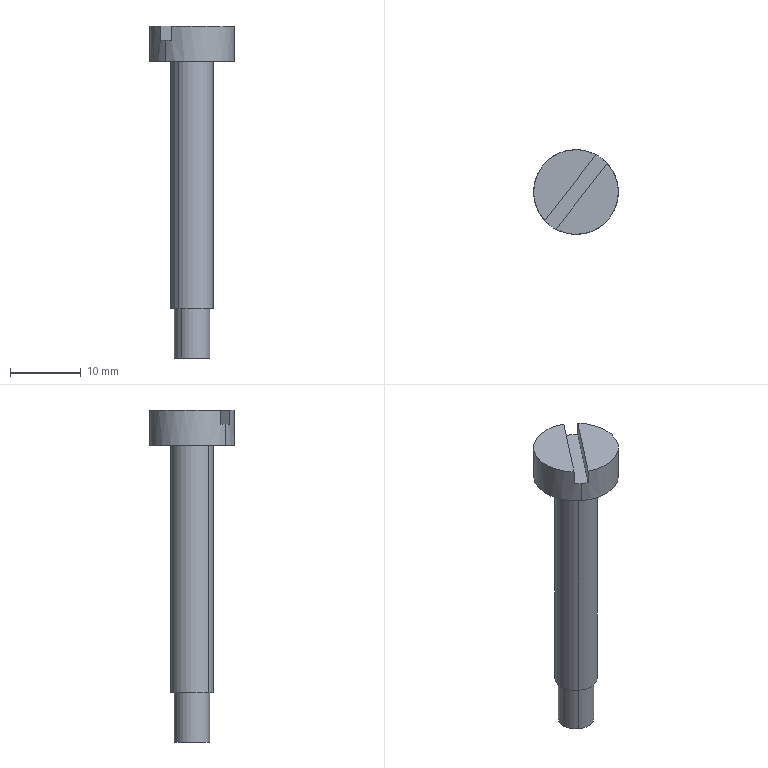Part | SolidWorks | features BaseBody 1 | 1 solid | 14 faces | box 12 x 12 x 47 mm | volume 1645 mm3 | plane 8 | cylinder 6 | commonest cylinder face diameters 5 x2 6 x2 12 x2
STEP:
#1=CARTESIAN_POINT('',(-805.971,723.012,538.482));
#2=VERTEX_POINT('',#1);
#3=CARTESIAN_POINT('',(-798.71,732.355,538.482));
#4=VERTEX_POINT('',#3);
#5=CARTESIAN_POINT('',(-805.971,723.012,538.482));
#6=DIRECTION('',(0.6136,0.7896,0.));
#7=VECTOR('',#6,1000.);
#8=LINE('',#5,#7);
#9=EDGE_CURVE('',#2,#4,#8,.T.);
#10=ORIENTED_EDGE('',*,*,#9,.F.);
#11=CARTESIAN_POINT('',(-805.971,723.012,540.482));
#12=VERTEX_POINT('',#11);
#13=CARTESIAN_POINT('',(-805.971,723.012,538.482));
#14=DIRECTION('',(0.,0.,1.));
#15=VECTOR('',#14,1000.);
#16=LINE('',#13,#15);
#17=EDGE_CURVE('',#2,#12,#16,.T.);
#18=ORIENTED_EDGE('',*,*,#17,.T.);
#19=CARTESIAN_POINT('',(-798.71,732.355,540.482));
#20=VERTEX_POINT('',#19);
#21=CARTESIAN_POINT('',(-798.71,732.355,540.482));
#22=DIRECTION('',(-0.6136,-0.7896,0.));
#23=VECTOR('',#22,1000.);
#24=LINE('',#21,#23);
#25=EDGE_CURVE('',#20,#12,#24,.T.);
#26=ORIENTED_EDGE('',*,*,#25,.F.);
#27=CARTESIAN_POINT('',(-798.71,732.355,540.482));
#28=DIRECTION('',(0.,0.,-1.));
#29=VECTOR('',#28,1000.);
#30=LINE('',#27,#29);
#31=EDGE_CURVE('',#20,#4,#30,.T.);
#32=ORIENTED_EDGE('',*,*,#31,.T.);
#33=EDGE_LOOP('',(#10,#18,#26,#32));
#34=FACE_OUTER_BOUND('',#33,.T.);
#35=CARTESIAN_POINT('',(-798.054,733.198,538.482));
#36=DIRECTION('',(0.7896,-0.6136,0.));
#37=DIRECTION('',(0.,0.,-1.));
#38=AXIS2_PLACEMENT_3D('',#35,#36,#37);
#39=PLANE('',#38);
#40=ADVANCED_FACE('',(#34),#39,.F.);
#41=CARTESIAN_POINT('',(-806.812,723.56,535.482));
#42=VERTEX_POINT('',#41);
#43=CARTESIAN_POINT('',(-799.448,733.035,535.482));
#44=VERTEX_POINT('',#43);
#45=CARTESIAN_POINT('',(-803.13,728.297,535.482));
#46=DIRECTION('',(0.,0.,1.));
#47=DIRECTION('',(-0.6136,-0.7896,0.));
#48=AXIS2_PLACEMENT_3D('',#45,#46,#47);
#49=CIRCLE('',#48,6.);
#50=EDGE_CURVE('',#42,#44,#49,.T.);
#51=ORIENTED_EDGE('',*,*,#50,.T.);
#52=CARTESIAN_POINT('',(-799.448,733.035,538.482));
#53=VERTEX_POINT('',#52);
#54=CARTESIAN_POINT('',(-799.448,733.035,538.482));
#55=DIRECTION('',(0.,0.,-1.));
#56=VECTOR('',#55,1000.);
#57=LINE('',#54,#56);
#58=EDGE_CURVE('',#53,#44,#57,.T.);
#59=ORIENTED_EDGE('',*,*,#58,.F.);
#60=CARTESIAN_POINT('',(-803.13,728.297,538.482));
#61=DIRECTION('',(0.,0.,-1.));
#62=DIRECTION('',(0.6136,0.7896,0.));
#63=AXIS2_PLACEMENT_3D('',#60,#61,#62);
#64=CIRCLE('',#63,6.);
#65=EDGE_CURVE('',#53,#4,#64,.T.);
#66=ORIENTED_EDGE('',*,*,#65,.T.);
#67=ORIENTED_EDGE('',*,*,#31,.F.);
#68=CARTESIAN_POINT('',(-803.13,728.297,540.482));
#69=DIRECTION('',(0.,0.,-1.));
#70=DIRECTION('',(0.7367,0.6763,0.));
#71=AXIS2_PLACEMENT_3D('',#68,#69,#70);
#72=CIRCLE('',#71,6.);
#73=EDGE_CURVE('',#20,#12,#72,.T.);
#74=ORIENTED_EDGE('',*,*,#73,.T.);
#75=ORIENTED_EDGE('',*,*,#17,.F.);
#76=CARTESIAN_POINT('',(-806.812,723.56,538.482));
#77=VERTEX_POINT('',#76);
#78=CARTESIAN_POINT('',(-803.13,728.297,538.482));
#79=DIRECTION('',(0.,0.,-1.));
#80=DIRECTION('',(-0.4735,-0.8808,0.));
#81=AXIS2_PLACEMENT_3D('',#78,#79,#80);
#82=CIRCLE('',#81,6.);
#83=EDGE_CURVE('',#2,#77,#82,.T.);
#84=ORIENTED_EDGE('',*,*,#83,.T.);
#85=CARTESIAN_POINT('',(-806.812,723.56,535.482));
#86=DIRECTION('',(0.,0.,1.));
#87=VECTOR('',#86,1000.);
#88=LINE('',#85,#87);
#89=EDGE_CURVE('',#42,#77,#88,.T.);
#90=ORIENTED_EDGE('',*,*,#89,.F.);
#91=EDGE_LOOP('',(#51,#59,#66,#67,#74,#75,#84,#90));
#92=FACE_OUTER_BOUND('',#91,.T.);
#93=CARTESIAN_POINT('',(-803.13,728.297,540.482));
#94=DIRECTION('',(0.,0.,-1.));
#95=DIRECTION('',(-0.6136,-0.7896,0.));
#96=AXIS2_PLACEMENT_3D('',#93,#94,#95);
#97=CYLINDRICAL_SURFACE('',#96,6.);
#98=ADVANCED_FACE('',(#92),#97,.T.);
#99=CARTESIAN_POINT('',(-807.55,724.239,540.482));
#100=VERTEX_POINT('',#99);
#101=CARTESIAN_POINT('',(-807.55,724.239,538.482));
#102=VERTEX_POINT('',#101);
#103=CARTESIAN_POINT('',(-807.55,724.239,540.482));
#104=DIRECTION('',(0.,0.,-1.));
#105=VECTOR('',#104,1000.);
#106=LINE('',#103,#105);
#107=EDGE_CURVE('',#100,#102,#106,.T.);
#108=ORIENTED_EDGE('',*,*,#107,.F.);
#109=CARTESIAN_POINT('',(-800.289,733.582,540.482));
#110=VERTEX_POINT('',#109);
#111=CARTESIAN_POINT('',(-803.13,728.297,540.482));
#112=DIRECTION('',(0.,0.,-1.));
#113=DIRECTION('',(-0.7367,-0.6763,0.));
#114=AXIS2_PLACEMENT_3D('',#111,#112,#113);
#115=CIRCLE('',#114,6.);
#116=EDGE_CURVE('',#100,#110,#115,.T.);
#117=ORIENTED_EDGE('',*,*,#116,.T.);
#118=CARTESIAN_POINT('',(-800.289,733.582,538.482));
#119=VERTEX_POINT('',#118);
#120=CARTESIAN_POINT('',(-800.289,733.582,538.482));
#121=DIRECTION('',(0.,0.,1.));
#122=VECTOR('',#121,1000.);
#123=LINE('',#120,#122);
#124=EDGE_CURVE('',#119,#110,#123,.T.);
#125=ORIENTED_EDGE('',*,*,#124,.F.);
#126=CARTESIAN_POINT('',(-803.13,728.297,538.482));
#127=DIRECTION('',(0.,0.,-1.));
#128=DIRECTION('',(0.4735,0.8808,0.));
#129=AXIS2_PLACEMENT_3D('',#126,#127,#128);
#130=CIRCLE('',#129,6.);
#131=EDGE_CURVE('',#119,#53,#130,.T.);
#132=ORIENTED_EDGE('',*,*,#131,.T.);
#133=ORIENTED_EDGE('',*,*,#58,.T.);
#134=CARTESIAN_POINT('',(-803.13,728.297,535.482));
#135=DIRECTION('',(0.,0.,1.));
#136=DIRECTION('',(0.6136,0.7896,0.));
#137=AXIS2_PLACEMENT_3D('',#134,#135,#136);
#138=CIRCLE('',#137,6.);
#139=EDGE_CURVE('',#44,#42,#138,.T.);
#140=ORIENTED_EDGE('',*,*,#139,.T.);
#141=ORIENTED_EDGE('',*,*,#89,.T.);
#142=CARTESIAN_POINT('',(-803.13,728.297,538.482));
#143=DIRECTION('',(0.,0.,-1.));
#144=DIRECTION('',(-0.6136,-0.7896,0.));
#145=AXIS2_PLACEMENT_3D('',#142,#143,#144);
#146=CIRCLE('',#145,6.);
#147=EDGE_CURVE('',#77,#102,#146,.T.);
#148=ORIENTED_EDGE('',*,*,#147,.T.);
#149=EDGE_LOOP('',(#108,#117,#125,#132,#133,#140,#141,#148));
#150=FACE_OUTER_BOUND('',#149,.T.);
#151=CARTESIAN_POINT('',(-803.13,728.297,540.482));
#152=DIRECTION('',(0.,0.,-1.));
#153=DIRECTION('',(-0.6136,-0.7896,0.));
#154=AXIS2_PLACEMENT_3D('',#151,#152,#153);
#155=CYLINDRICAL_SURFACE('',#154,6.);
#156=ADVANCED_FACE('',(#150),#155,.T.);
#157=CARTESIAN_POINT('',(-807.55,724.239,538.482));
#158=DIRECTION('',(0.6136,0.7896,0.));
#159=VECTOR('',#158,1000.);
#160=LINE('',#157,#159);
#161=EDGE_CURVE('',#102,#119,#160,.T.);
#162=ORIENTED_EDGE('',*,*,#161,.F.);
#163=ORIENTED_EDGE('',*,*,#147,.F.);
#164=ORIENTED_EDGE('',*,*,#83,.F.);
#165=ORIENTED_EDGE('',*,*,#9,.T.);
#166=ORIENTED_EDGE('',*,*,#65,.F.);
#167=ORIENTED_EDGE('',*,*,#131,.F.);
#168=EDGE_LOOP('',(#162,#163,#164,#165,#166,#167));
#169=FACE_OUTER_BOUND('',#168,.T.);
#170=CARTESIAN_POINT('',(-803.13,728.297,538.482));
#171=DIRECTION('',(0.,0.,1.));
#172=DIRECTION('',(0.6136,0.7896,0.));
#173=AXIS2_PLACEMENT_3D('',#170,#171,#172);
#174=PLANE('',#173);
#175=ADVANCED_FACE('',(#169),#174,.T.);
#176=ORIENTED_EDGE('',*,*,#161,.T.);
#177=ORIENTED_EDGE('',*,*,#124,.T.);
#178=CARTESIAN_POINT('',(-807.55,724.239,540.482));
#179=DIRECTION('',(0.6136,0.7896,0.));
#180=VECTOR('',#179,1000.);
#181=LINE('',#178,#180);
#182=EDGE_CURVE('',#100,#110,#181,.T.);
#183=ORIENTED_EDGE('',*,*,#182,.F.);
#184=ORIENTED_EDGE('',*,*,#107,.T.);
#185=EDGE_LOOP('',(#176,#177,#183,#184));
#186=FACE_OUTER_BOUND('',#185,.T.);
#187=CARTESIAN_POINT('',(-799.634,734.425,538.482));
#188=DIRECTION('',(-0.7896,0.6136,0.));
#189=DIRECTION('',(0.,0.,1.));
#190=AXIS2_PLACEMENT_3D('',#187,#188,#189);
#191=PLANE('',#190);
#192=ADVANCED_FACE('',(#186),#191,.F.);
#193=ORIENTED_EDGE('',*,*,#182,.T.);
#194=ORIENTED_EDGE('',*,*,#116,.F.);
#195=EDGE_LOOP('',(#193,#194));
#196=FACE_OUTER_BOUND('',#195,.T.);
#197=CARTESIAN_POINT('',(-803.13,728.297,540.482));
#198=DIRECTION('',(0.,0.,1.));
#199=DIRECTION('',(0.6136,0.7896,0.));
#200=AXIS2_PLACEMENT_3D('',#197,#198,#199);
#201=PLANE('',#200);
#202=ADVANCED_FACE('',(#196),#201,.T.);
#203=ORIENTED_EDGE('',*,*,#139,.F.);
#204=ORIENTED_EDGE('',*,*,#50,.F.);
#205=EDGE_LOOP('',(#203,#204));
#206=FACE_OUTER_BOUND('',#205,.T.);
#207=CARTESIAN_POINT('',(-804.971,725.928,535.482));
#208=VERTEX_POINT('',#207);
#209=CARTESIAN_POINT('',(-801.289,730.666,535.482));
#210=VERTEX_POINT('',#209);
#211=CARTESIAN_POINT('',(-803.13,728.297,535.482));
#212=DIRECTION('',(0.,0.,-1.));
#213=DIRECTION('',(-0.6136,-0.7896,0.));
#214=AXIS2_PLACEMENT_3D('',#211,#212,#213);
#215=CIRCLE('',#214,3.);
#216=EDGE_CURVE('',#208,#210,#215,.T.);
#217=ORIENTED_EDGE('',*,*,#216,.F.);
#218=CARTESIAN_POINT('',(-803.13,728.297,535.482));
#219=DIRECTION('',(0.,0.,-1.));
#220=DIRECTION('',(0.6136,0.7896,0.));
#221=AXIS2_PLACEMENT_3D('',#218,#219,#220);
#222=CIRCLE('',#221,3.);
#223=EDGE_CURVE('',#210,#208,#222,.T.);
#224=ORIENTED_EDGE('',*,*,#223,.F.);
#225=EDGE_LOOP('',(#217,#224));
#226=FACE_BOUND('',#225,.T.);
#227=CARTESIAN_POINT('',(-803.13,728.297,535.482));
#228=DIRECTION('',(0.,0.,1.));
#229=DIRECTION('',(0.6136,0.7896,0.));
#230=AXIS2_PLACEMENT_3D('',#227,#228,#229);
#231=PLANE('',#230);
#232=ADVANCED_FACE('',(#206,#226),#231,.F.);
#233=CARTESIAN_POINT('',(-804.971,725.928,500.482));
#234=VERTEX_POINT('',#233);
#235=CARTESIAN_POINT('',(-804.971,725.928,535.482));
#236=DIRECTION('',(0.,0.,-1.));
#237=VECTOR('',#236,1000.);
#238=LINE('',#235,#237);
#239=EDGE_CURVE('',#208,#234,#238,.T.);
#240=ORIENTED_EDGE('',*,*,#239,.T.);
#241=CARTESIAN_POINT('',(-801.289,730.666,500.482));
#242=VERTEX_POINT('',#241);
#243=CARTESIAN_POINT('',(-803.13,728.297,500.482));
#244=DIRECTION('',(0.,0.,1.));
#245=DIRECTION('',(-0.6136,-0.7896,0.));
#246=AXIS2_PLACEMENT_3D('',#243,#244,#245);
#247=CIRCLE('',#246,3.);
#248=EDGE_CURVE('',#234,#242,#247,.T.);
#249=ORIENTED_EDGE('',*,*,#248,.T.);
#250=CARTESIAN_POINT('',(-801.289,730.666,500.482));
#251=DIRECTION('',(0.,0.,1.));
#252=VECTOR('',#251,1000.);
#253=LINE('',#250,#252);
#254=EDGE_CURVE('',#242,#210,#253,.T.);
#255=ORIENTED_EDGE('',*,*,#254,.T.);
#256=ORIENTED_EDGE('',*,*,#223,.T.);
#257=EDGE_LOOP('',(#240,#249,#255,#256));
#258=FACE_OUTER_BOUND('',#257,.T.);
#259=CARTESIAN_POINT('',(-803.13,728.297,503.482));
#260=DIRECTION('',(0.,0.,-1.));
#261=DIRECTION('',(-0.6136,-0.7896,0.));
#262=AXIS2_PLACEMENT_3D('',#259,#260,#261);
#263=CYLINDRICAL_SURFACE('',#262,3.);
#264=ADVANCED_FACE('',(#258),#263,.T.);
#265=ORIENTED_EDGE('',*,*,#254,.F.);
#266=CARTESIAN_POINT('',(-803.13,728.297,500.482));
#267=DIRECTION('',(0.,0.,1.));
#268=DIRECTION('',(0.6136,0.7896,0.));
#269=AXIS2_PLACEMENT_3D('',#266,#267,#268);
#270=CIRCLE('',#269,3.);
#271=EDGE_CURVE('',#242,#234,#270,.T.);
#272=ORIENTED_EDGE('',*,*,#271,.T.);
#273=ORIENTED_EDGE('',*,*,#239,.F.);
#274=ORIENTED_EDGE('',*,*,#216,.T.);
#275=EDGE_LOOP('',(#265,#272,#273,#274));
#276=FACE_OUTER_BOUND('',#275,.T.);
#277=CARTESIAN_POINT('',(-803.13,728.297,503.482));
#278=DIRECTION('',(0.,0.,-1.));
#279=DIRECTION('',(-0.6136,-0.7896,0.));
#280=AXIS2_PLACEMENT_3D('',#277,#278,#279);
#281=CYLINDRICAL_SURFACE('',#280,3.);
#282=ADVANCED_FACE('',(#276),#281,.T.);
#283=ORIENTED_EDGE('',*,*,#248,.F.);
#284=ORIENTED_EDGE('',*,*,#271,.F.);
#285=EDGE_LOOP('',(#283,#284));
#286=FACE_OUTER_BOUND('',#285,.T.);
#287=CARTESIAN_POINT('',(-804.664,726.323,500.482));
#288=VERTEX_POINT('',#287);
#289=CARTESIAN_POINT('',(-801.596,730.271,500.482));
#290=VERTEX_POINT('',#289);
#291=CARTESIAN_POINT('',(-803.13,728.297,500.482));
#292=DIRECTION('',(0.,0.,-1.));
#293=DIRECTION('',(-0.6136,-0.7896,0.));
#294=AXIS2_PLACEMENT_3D('',#291,#292,#293);
#295=CIRCLE('',#294,2.5);
#296=EDGE_CURVE('',#288,#290,#295,.T.);
#297=ORIENTED_EDGE('',*,*,#296,.F.);
#298=CARTESIAN_POINT('',(-803.13,728.297,500.482));
#299=DIRECTION('',(0.,0.,-1.));
#300=DIRECTION('',(0.6136,0.7896,0.));
#301=AXIS2_PLACEMENT_3D('',#298,#299,#300);
#302=CIRCLE('',#301,2.5);
#303=EDGE_CURVE('',#290,#288,#302,.T.);
#304=ORIENTED_EDGE('',*,*,#303,.F.);
#305=EDGE_LOOP('',(#297,#304));
#306=FACE_BOUND('',#305,.T.);
#307=CARTESIAN_POINT('',(-803.13,728.297,500.482));
#308=DIRECTION('',(0.,0.,-1.));
#309=DIRECTION('',(-0.6136,-0.7896,0.));
#310=AXIS2_PLACEMENT_3D('',#307,#308,#309);
#311=PLANE('',#310);
#312=ADVANCED_FACE('',(#286,#306),#311,.T.);
#313=CARTESIAN_POINT('',(-804.664,726.323,493.482));
#314=VERTEX_POINT('',#313);
#315=CARTESIAN_POINT('',(-801.596,730.271,493.482));
#316=VERTEX_POINT('',#315);
#317=CARTESIAN_POINT('',(-803.13,728.297,493.482));
#318=DIRECTION('',(0.,0.,1.));
#319=DIRECTION('',(-0.6136,-0.7896,0.));
#320=AXIS2_PLACEMENT_3D('',#317,#318,#319);
#321=CIRCLE('',#320,2.5);
#322=EDGE_CURVE('',#314,#316,#321,.T.);
#323=ORIENTED_EDGE('',*,*,#322,.T.);
#324=CARTESIAN_POINT('',(-801.596,730.271,493.482));
#325=DIRECTION('',(0.,0.,1.));
#326=VECTOR('',#325,1000.);
#327=LINE('',#324,#326);
#328=EDGE_CURVE('',#316,#290,#327,.T.);
#329=ORIENTED_EDGE('',*,*,#328,.T.);
#330=ORIENTED_EDGE('',*,*,#303,.T.);
#331=CARTESIAN_POINT('',(-804.664,726.323,500.482));
#332=DIRECTION('',(0.,0.,-1.));
#333=VECTOR('',#332,1000.);
#334=LINE('',#331,#333);
#335=EDGE_CURVE('',#288,#314,#334,.T.);
#336=ORIENTED_EDGE('',*,*,#335,.T.);
#337=EDGE_LOOP('',(#323,#329,#330,#336));
#338=FACE_OUTER_BOUND('',#337,.T.);
#339=CARTESIAN_POINT('',(-803.13,728.297,493.482));
#340=DIRECTION('',(0.,0.,1.));
#341=DIRECTION('',(0.6136,0.7896,0.));
#342=AXIS2_PLACEMENT_3D('',#339,#340,#341);
#343=CYLINDRICAL_SURFACE('',#342,2.5);
#344=ADVANCED_FACE('',(#338),#343,.T.);
#345=CARTESIAN_POINT('',(-803.13,728.297,493.482));
#346=DIRECTION('',(0.,0.,1.));
#347=DIRECTION('',(0.6136,0.7896,0.));
#348=AXIS2_PLACEMENT_3D('',#345,#346,#347);
#349=CIRCLE('',#348,2.5);
#350=EDGE_CURVE('',#316,#314,#349,.T.);
#351=ORIENTED_EDGE('',*,*,#350,.T.);
#352=ORIENTED_EDGE('',*,*,#335,.F.);
#353=ORIENTED_EDGE('',*,*,#296,.T.);
#354=ORIENTED_EDGE('',*,*,#328,.F.);
#355=EDGE_LOOP('',(#351,#352,#353,#354));
#356=FACE_OUTER_BOUND('',#355,.T.);
#357=CARTESIAN_POINT('',(-803.13,728.297,493.482));
#358=DIRECTION('',(0.,0.,1.));
#359=DIRECTION('',(0.6136,0.7896,0.));
#360=AXIS2_PLACEMENT_3D('',#357,#358,#359);
#361=CYLINDRICAL_SURFACE('',#360,2.5);
#362=ADVANCED_FACE('',(#356),#361,.T.);
#363=ORIENTED_EDGE('',*,*,#350,.F.);
#364=ORIENTED_EDGE('',*,*,#322,.F.);
#365=EDGE_LOOP('',(#363,#364));
#366=FACE_OUTER_BOUND('',#365,.T.);
#367=CARTESIAN_POINT('',(-803.13,728.297,493.482));
#368=DIRECTION('',(0.,0.,-1.));
#369=DIRECTION('',(-0.6136,-0.7896,0.));
#370=AXIS2_PLACEMENT_3D('',#367,#368,#369);
#371=PLANE('',#370);
#372=ADVANCED_FACE('',(#366),#371,.T.);
#373=ORIENTED_EDGE('',*,*,#25,.T.);
#374=ORIENTED_EDGE('',*,*,#73,.F.);
#375=EDGE_LOOP('',(#373,#374));
#376=FACE_OUTER_BOUND('',#375,.T.);
#377=CARTESIAN_POINT('',(-803.13,728.297,540.482));
#378=DIRECTION('',(0.,0.,1.));
#379=DIRECTION('',(0.6136,0.7896,0.));
#380=AXIS2_PLACEMENT_3D('',#377,#378,#379);
#381=PLANE('',#380);
#382=ADVANCED_FACE('',(#376),#381,.T.);
#383=CLOSED_SHELL('',(#40,#98,#156,#175,#192,#202,#232,#264,#282,#312,#344,#362,#372,#382));
#384=MANIFOLD_SOLID_BREP('',#383);
#385=CARTESIAN_POINT('',(0.,0.,0.));
#386=DIRECTION('',(0.,0.,1.));
#387=DIRECTION('',(1.,0.,0.));
#388=AXIS2_PLACEMENT_3D('',#385,#386,#387);
#389=(LENGTH_UNIT()NAMED_UNIT(*)SI_UNIT(.MILLI.,.METRE.));
#390=UNCERTAINTY_MEASURE_WITH_UNIT(LENGTH_MEASURE(0.00001),#389,'','');
#391=(NAMED_UNIT(*)PLANE_ANGLE_UNIT()SI_UNIT($,.RADIAN.));
#392=(NAMED_UNIT(*)SI_UNIT($,.STERADIAN.)SOLID_ANGLE_UNIT());
#393=(GEOMETRIC_REPRESENTATION_CONTEXT(3)GLOBAL_UNCERTAINTY_ASSIGNED_CONTEXT((#390))GLOBAL_UNIT_ASSIGNED_CONTEXT((#389,#391,#392))REPRESENTATION_CONTEXT('',''));
#394=ADVANCED_BREP_SHAPE_REPRESENTATION('',(#384,#388),#393);